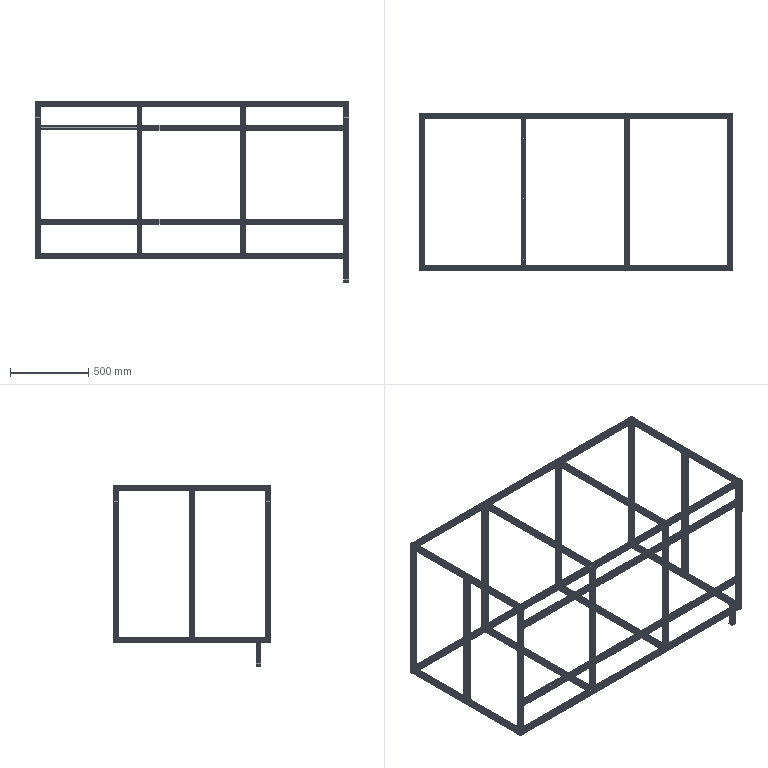Part | SolidWorks | 29 solids | 2220 faces | box 2000 x 1000 x 1150 mm | volume 9577291 mm3 | plane 1414 | cylinder 806 | commonest cylinder face diameters 11 x240 4.2 x232 6.6 x160 4 x116 6.8 x58